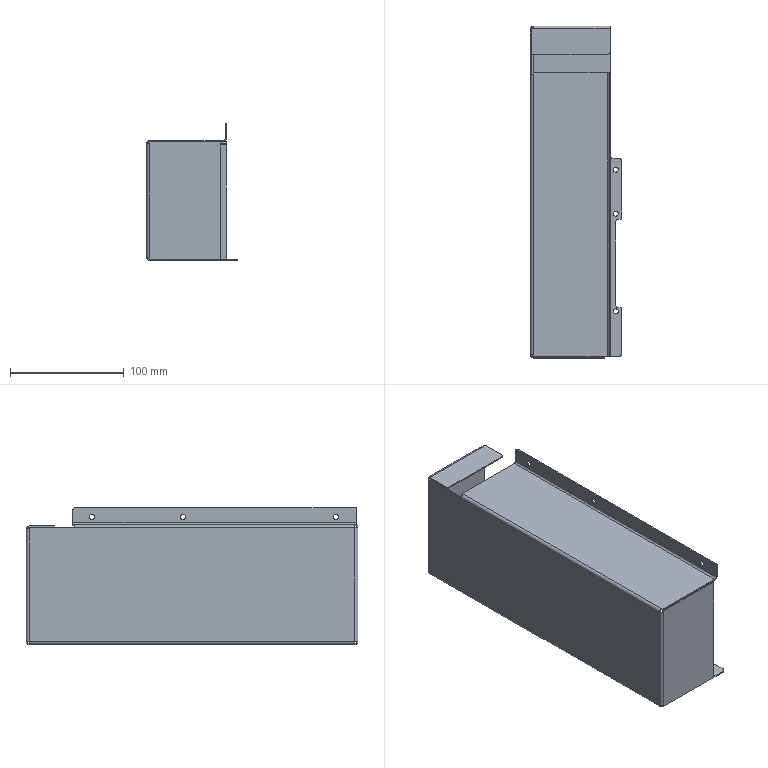Part | NX | 1 solid | 96 faces | box 80 x 291.5 x 120 mm | volume 87007 mm3 | plane 52 | cylinder 32 | cone 12 | commonest cylinder face diameters 4.5 x12 5 x8 3.2 x6 5.2 x6